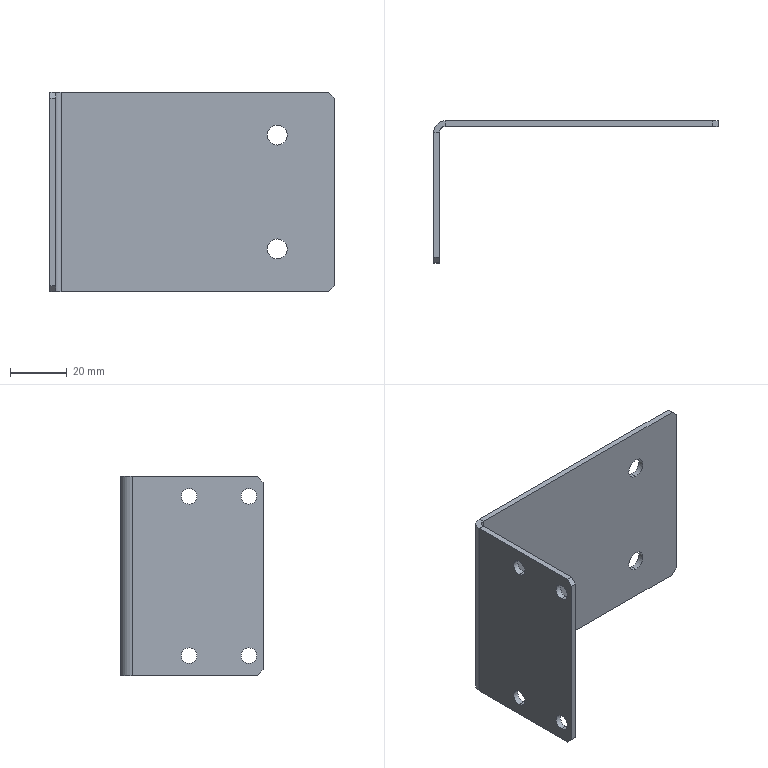Part | NX | features BREP 1 | 1 solid | 30 faces | box 100 x 50 x 70 mm | volume 20180 mm3 | plane 16 | cylinder 14 | commonest cylinder face diameters 5.5 x8 7 x4 4 x1 8 x1
STEP:
#1=CARTESIAN_POINT('',(-98.,-50.,-33.));
#2=VERTEX_POINT('',#1);
#3=CARTESIAN_POINT('',(-98.,-48.,-35.));
#4=VERTEX_POINT('',#3);
#5=CARTESIAN_POINT('',(-98.,-59.,-24.));
#6=DIRECTION('',(0.,0.7071,-0.7071));
#7=VECTOR('',#6,1000.);
#8=LINE('',#5,#7);
#9=EDGE_CURVE('',#2,#4,#8,.T.);
#10=ORIENTED_EDGE('',*,*,#9,.F.);
#11=CARTESIAN_POINT('',(-100.,-50.,-33.));
#12=VERTEX_POINT('',#11);
#13=CARTESIAN_POINT('',(-98.,-50.,-33.));
#14=DIRECTION('',(1.,0.,0.));
#15=VECTOR('',#14,1000.);
#16=LINE('',#13,#15);
#17=EDGE_CURVE('',#12,#2,#16,.T.);
#18=ORIENTED_EDGE('',*,*,#17,.F.);
#19=CARTESIAN_POINT('',(-100.,-48.,-35.));
#20=VERTEX_POINT('',#19);
#21=CARTESIAN_POINT('',(-100.,-48.,-35.));
#22=DIRECTION('',(0.,-0.7071,0.7071));
#23=VECTOR('',#22,1000.);
#24=LINE('',#21,#23);
#25=EDGE_CURVE('',#20,#12,#24,.T.);
#26=ORIENTED_EDGE('',*,*,#25,.F.);
#27=CARTESIAN_POINT('',(-96.,-48.,-35.));
#28=DIRECTION('',(-1.,0.,0.));
#29=VECTOR('',#28,1000.);
#30=LINE('',#27,#29);
#31=EDGE_CURVE('',#4,#20,#30,.T.);
#32=ORIENTED_EDGE('',*,*,#31,.F.);
#33=EDGE_LOOP('',(#10,#18,#26,#32));
#34=FACE_BOUND('',#33,.T.);
#35=CARTESIAN_POINT('',(-96.,-48.,-35.));
#36=DIRECTION('',(0.,0.7071,0.7071));
#37=DIRECTION('',(-1.,0.,0.));
#38=AXIS2_PLACEMENT_3D('',#35,#36,#37);
#39=PLANE('',#38);
#40=ADVANCED_FACE('',(#34),#39,.F.);
#41=CARTESIAN_POINT('',(-98.,-48.,35.));
#42=VERTEX_POINT('',#41);
#43=CARTESIAN_POINT('',(-98.,-50.,33.));
#44=VERTEX_POINT('',#43);
#45=CARTESIAN_POINT('',(-98.,-24.,59.));
#46=DIRECTION('',(0.,-0.7071,-0.7071));
#47=VECTOR('',#46,1000.);
#48=LINE('',#45,#47);
#49=EDGE_CURVE('',#42,#44,#48,.T.);
#50=ORIENTED_EDGE('',*,*,#49,.F.);
#51=CARTESIAN_POINT('',(-100.,-48.,35.));
#52=VERTEX_POINT('',#51);
#53=CARTESIAN_POINT('',(-96.,-48.,35.));
#54=DIRECTION('',(1.,0.,0.));
#55=VECTOR('',#54,1000.);
#56=LINE('',#53,#55);
#57=EDGE_CURVE('',#52,#42,#56,.T.);
#58=ORIENTED_EDGE('',*,*,#57,.F.);
#59=CARTESIAN_POINT('',(-100.,-50.,33.));
#60=VERTEX_POINT('',#59);
#61=CARTESIAN_POINT('',(-100.,-50.,33.));
#62=DIRECTION('',(0.,0.7071,0.7071));
#63=VECTOR('',#62,1000.);
#64=LINE('',#61,#63);
#65=EDGE_CURVE('',#60,#52,#64,.T.);
#66=ORIENTED_EDGE('',*,*,#65,.F.);
#67=CARTESIAN_POINT('',(-98.,-50.,33.));
#68=DIRECTION('',(-1.,0.,0.));
#69=VECTOR('',#68,1000.);
#70=LINE('',#67,#69);
#71=EDGE_CURVE('',#44,#60,#70,.T.);
#72=ORIENTED_EDGE('',*,*,#71,.F.);
#73=EDGE_LOOP('',(#50,#58,#66,#72));
#74=FACE_BOUND('',#73,.T.);
#75=CARTESIAN_POINT('',(-98.,-50.,33.));
#76=DIRECTION('',(0.,0.7071,-0.7071));
#77=DIRECTION('',(-1.,0.,0.));
#78=AXIS2_PLACEMENT_3D('',#75,#76,#77);
#79=PLANE('',#78);
#80=ADVANCED_FACE('',(#74),#79,.F.);
#81=CARTESIAN_POINT('',(0.,0.,-33.));
#82=VERTEX_POINT('',#81);
#83=CARTESIAN_POINT('',(-2.,0.,-35.));
#84=VERTEX_POINT('',#83);
#85=CARTESIAN_POINT('',(-2.,0.,-35.));
#86=DIRECTION('',(-0.7071,0.,-0.7071));
#87=VECTOR('',#86,1000.);
#88=LINE('',#85,#87);
#89=EDGE_CURVE('',#82,#84,#88,.T.);
#90=ORIENTED_EDGE('',*,*,#89,.F.);
#91=CARTESIAN_POINT('',(0.,-2.,-33.));
#92=VERTEX_POINT('',#91);
#93=CARTESIAN_POINT('',(0.,0.,-33.));
#94=DIRECTION('',(0.,1.,0.));
#95=VECTOR('',#94,1000.);
#96=LINE('',#93,#95);
#97=EDGE_CURVE('',#92,#82,#96,.T.);
#98=ORIENTED_EDGE('',*,*,#97,.F.);
#99=CARTESIAN_POINT('',(-2.,-2.,-35.));
#100=VERTEX_POINT('',#99);
#101=CARTESIAN_POINT('',(34.,-2.,1.));
#102=DIRECTION('',(0.7071,0.,0.7071));
#103=VECTOR('',#102,1000.);
#104=LINE('',#101,#103);
#105=EDGE_CURVE('',#100,#92,#104,.T.);
#106=ORIENTED_EDGE('',*,*,#105,.F.);
#107=CARTESIAN_POINT('',(-2.,-2.,-35.));
#108=DIRECTION('',(0.,-1.,0.));
#109=VECTOR('',#108,1000.);
#110=LINE('',#107,#109);
#111=EDGE_CURVE('',#84,#100,#110,.T.);
#112=ORIENTED_EDGE('',*,*,#111,.F.);
#113=EDGE_LOOP('',(#90,#98,#106,#112));
#114=FACE_BOUND('',#113,.T.);
#115=CARTESIAN_POINT('',(-2.,-4.,-35.));
#116=DIRECTION('',(0.7071,0.,-0.7071));
#117=DIRECTION('',(0.,1.,0.));
#118=AXIS2_PLACEMENT_3D('',#115,#116,#117);
#119=PLANE('',#118);
#120=ADVANCED_FACE('',(#114),#119,.T.);
#121=CARTESIAN_POINT('',(-2.,0.,35.));
#122=VERTEX_POINT('',#121);
#123=CARTESIAN_POINT('',(0.,0.,33.));
#124=VERTEX_POINT('',#123);
#125=CARTESIAN_POINT('',(0.,0.,33.));
#126=DIRECTION('',(0.7071,0.,-0.7071));
#127=VECTOR('',#126,1000.);
#128=LINE('',#125,#127);
#129=EDGE_CURVE('',#122,#124,#128,.T.);
#130=ORIENTED_EDGE('',*,*,#129,.F.);
#131=CARTESIAN_POINT('',(-2.,-2.,35.));
#132=VERTEX_POINT('',#131);
#133=CARTESIAN_POINT('',(-2.,-4.,35.));
#134=DIRECTION('',(0.,1.,0.));
#135=VECTOR('',#134,1000.);
#136=LINE('',#133,#135);
#137=EDGE_CURVE('',#132,#122,#136,.T.);
#138=ORIENTED_EDGE('',*,*,#137,.F.);
#139=CARTESIAN_POINT('',(0.,-2.,33.));
#140=VERTEX_POINT('',#139);
#141=CARTESIAN_POINT('',(-1.,-2.,34.));
#142=DIRECTION('',(-0.7071,0.,0.7071));
#143=VECTOR('',#142,1000.);
#144=LINE('',#141,#143);
#145=EDGE_CURVE('',#140,#132,#144,.T.);
#146=ORIENTED_EDGE('',*,*,#145,.F.);
#147=CARTESIAN_POINT('',(0.,0.,33.));
#148=DIRECTION('',(0.,-1.,0.));
#149=VECTOR('',#148,1000.);
#150=LINE('',#147,#149);
#151=EDGE_CURVE('',#124,#140,#150,.T.);
#152=ORIENTED_EDGE('',*,*,#151,.F.);
#153=EDGE_LOOP('',(#130,#138,#146,#152));
#154=FACE_BOUND('',#153,.T.);
#155=CARTESIAN_POINT('',(0.,0.,33.));
#156=DIRECTION('',(-0.7071,0.,-0.7071));
#157=DIRECTION('',(0.,-1.,0.));
#158=AXIS2_PLACEMENT_3D('',#155,#156,#157);
#159=PLANE('',#158);
#160=ADVANCED_FACE('',(#154),#159,.F.);
#161=CARTESIAN_POINT('',(-20.,0.,-23.5));
#162=VERTEX_POINT('',#161);
#163=CARTESIAN_POINT('',(-20.,-2.,-23.5));
#164=VERTEX_POINT('',#163);
#165=CARTESIAN_POINT('',(-20.,0.,-23.5));
#166=DIRECTION('',(0.,1.,0.));
#167=VECTOR('',#166,1000.);
#168=LINE('',#165,#167);
#169=EDGE_CURVE('',#162,#164,#168,.F.);
#170=ORIENTED_EDGE('',*,*,#169,.T.);
#171=CARTESIAN_POINT('',(-20.,-2.,-16.5));
#172=VERTEX_POINT('',#171);
#173=CARTESIAN_POINT('',(-20.,-2.,-20.));
#174=DIRECTION('',(0.,-1.,0.));
#175=DIRECTION('',(1.,0.,0.));
#176=AXIS2_PLACEMENT_3D('',#173,#174,#175);
#177=CIRCLE('',#176,3.5);
#178=EDGE_CURVE('',#164,#172,#177,.T.);
#179=ORIENTED_EDGE('',*,*,#178,.T.);
#180=CARTESIAN_POINT('',(-20.,0.,-16.5));
#181=VERTEX_POINT('',#180);
#182=CARTESIAN_POINT('',(-20.,0.,-16.5));
#183=DIRECTION('',(0.,1.,0.));
#184=VECTOR('',#183,1000.);
#185=LINE('',#182,#184);
#186=EDGE_CURVE('',#181,#172,#185,.F.);
#187=ORIENTED_EDGE('',*,*,#186,.F.);
#188=CARTESIAN_POINT('',(-20.,0.,-20.));
#189=DIRECTION('',(0.,1.,0.));
#190=DIRECTION('',(0.,0.,1.));
#191=AXIS2_PLACEMENT_3D('',#188,#189,#190);
#192=CIRCLE('',#191,3.5);
#193=EDGE_CURVE('',#181,#162,#192,.T.);
#194=ORIENTED_EDGE('',*,*,#193,.T.);
#195=EDGE_LOOP('',(#170,#179,#187,#194));
#196=FACE_BOUND('',#195,.T.);
#197=CARTESIAN_POINT('',(-20.,0.,-20.));
#198=DIRECTION('',(0.,1.,0.));
#199=DIRECTION('',(0.,0.,1.));
#200=AXIS2_PLACEMENT_3D('',#197,#198,#199);
#201=CYLINDRICAL_SURFACE('',#200,3.5);
#202=ADVANCED_FACE('',(#196),#201,.F.);
#203=CARTESIAN_POINT('',(-20.,0.,16.5));
#204=VERTEX_POINT('',#203);
#205=CARTESIAN_POINT('',(-20.,-2.,16.5));
#206=VERTEX_POINT('',#205);
#207=CARTESIAN_POINT('',(-20.,0.,16.5));
#208=DIRECTION('',(0.,1.,0.));
#209=VECTOR('',#208,1000.);
#210=LINE('',#207,#209);
#211=EDGE_CURVE('',#204,#206,#210,.F.);
#212=ORIENTED_EDGE('',*,*,#211,.T.);
#213=CARTESIAN_POINT('',(-20.,-2.,23.5));
#214=VERTEX_POINT('',#213);
#215=CARTESIAN_POINT('',(-20.,-2.,20.));
#216=DIRECTION('',(0.,-1.,0.));
#217=DIRECTION('',(1.,0.,0.));
#218=AXIS2_PLACEMENT_3D('',#215,#216,#217);
#219=CIRCLE('',#218,3.5);
#220=EDGE_CURVE('',#206,#214,#219,.T.);
#221=ORIENTED_EDGE('',*,*,#220,.T.);
#222=CARTESIAN_POINT('',(-20.,0.,23.5));
#223=VERTEX_POINT('',#222);
#224=CARTESIAN_POINT('',(-20.,0.,23.5));
#225=DIRECTION('',(0.,1.,0.));
#226=VECTOR('',#225,1000.);
#227=LINE('',#224,#226);
#228=EDGE_CURVE('',#223,#214,#227,.F.);
#229=ORIENTED_EDGE('',*,*,#228,.F.);
#230=CARTESIAN_POINT('',(-20.,0.,20.));
#231=DIRECTION('',(0.,1.,0.));
#232=DIRECTION('',(0.,0.,1.));
#233=AXIS2_PLACEMENT_3D('',#230,#231,#232);
#234=CIRCLE('',#233,3.5);
#235=EDGE_CURVE('',#223,#204,#234,.T.);
#236=ORIENTED_EDGE('',*,*,#235,.T.);
#237=EDGE_LOOP('',(#212,#221,#229,#236));
#238=FACE_BOUND('',#237,.T.);
#239=CARTESIAN_POINT('',(-20.,0.,20.));
#240=DIRECTION('',(0.,1.,0.));
#241=DIRECTION('',(0.,0.,1.));
#242=AXIS2_PLACEMENT_3D('',#239,#240,#241);
#243=CYLINDRICAL_SURFACE('',#242,3.5);
#244=ADVANCED_FACE('',(#238),#243,.F.);
#245=CARTESIAN_POINT('',(-100.,-24.,-30.75));
#246=VERTEX_POINT('',#245);
#247=CARTESIAN_POINT('',(-98.,-24.,-30.75));
#248=VERTEX_POINT('',#247);
#249=CARTESIAN_POINT('',(-100.,-24.,-30.75));
#250=DIRECTION('',(-1.,0.,0.));
#251=VECTOR('',#250,1000.);
#252=LINE('',#249,#251);
#253=EDGE_CURVE('',#246,#248,#252,.F.);
#254=ORIENTED_EDGE('',*,*,#253,.T.);
#255=CARTESIAN_POINT('',(-98.,-24.,-25.25));
#256=VERTEX_POINT('',#255);
#257=CARTESIAN_POINT('',(-98.,-24.,-28.));
#258=DIRECTION('',(1.,0.,0.));
#259=DIRECTION('',(0.,0.,-1.));
#260=AXIS2_PLACEMENT_3D('',#257,#258,#259);
#261=CIRCLE('',#260,2.75);
#262=EDGE_CURVE('',#248,#256,#261,.T.);
#263=ORIENTED_EDGE('',*,*,#262,.T.);
#264=CARTESIAN_POINT('',(-100.,-24.,-25.25));
#265=VERTEX_POINT('',#264);
#266=CARTESIAN_POINT('',(-100.,-24.,-25.25));
#267=DIRECTION('',(-1.,0.,0.));
#268=VECTOR('',#267,1000.);
#269=LINE('',#266,#268);
#270=EDGE_CURVE('',#265,#256,#269,.F.);
#271=ORIENTED_EDGE('',*,*,#270,.F.);
#272=CARTESIAN_POINT('',(-100.,-24.,-28.));
#273=DIRECTION('',(-1.,0.,0.));
#274=DIRECTION('',(0.,0.,1.));
#275=AXIS2_PLACEMENT_3D('',#272,#273,#274);
#276=CIRCLE('',#275,2.75);
#277=EDGE_CURVE('',#265,#246,#276,.T.);
#278=ORIENTED_EDGE('',*,*,#277,.T.);
#279=EDGE_LOOP('',(#254,#263,#271,#278));
#280=FACE_BOUND('',#279,.T.);
#281=CARTESIAN_POINT('',(-100.,-24.,-28.));
#282=DIRECTION('',(-1.,0.,0.));
#283=DIRECTION('',(0.,0.,1.));
#284=AXIS2_PLACEMENT_3D('',#281,#282,#283);
#285=CYLINDRICAL_SURFACE('',#284,2.75);
#286=ADVANCED_FACE('',(#280),#285,.F.);
#287=CARTESIAN_POINT('',(-100.,-24.,25.25));
#288=VERTEX_POINT('',#287);
#289=CARTESIAN_POINT('',(-98.,-24.,25.25));
#290=VERTEX_POINT('',#289);
#291=CARTESIAN_POINT('',(-100.,-24.,25.25));
#292=DIRECTION('',(-1.,0.,0.));
#293=VECTOR('',#292,1000.);
#294=LINE('',#291,#293);
#295=EDGE_CURVE('',#288,#290,#294,.F.);
#296=ORIENTED_EDGE('',*,*,#295,.T.);
#297=CARTESIAN_POINT('',(-98.,-24.,30.75));
#298=VERTEX_POINT('',#297);
#299=CARTESIAN_POINT('',(-98.,-24.,28.));
#300=DIRECTION('',(1.,0.,0.));
#301=DIRECTION('',(0.,0.,-1.));
#302=AXIS2_PLACEMENT_3D('',#299,#300,#301);
#303=CIRCLE('',#302,2.75);
#304=EDGE_CURVE('',#290,#298,#303,.T.);
#305=ORIENTED_EDGE('',*,*,#304,.T.);
#306=CARTESIAN_POINT('',(-100.,-24.,30.75));
#307=VERTEX_POINT('',#306);
#308=CARTESIAN_POINT('',(-100.,-24.,30.75));
#309=DIRECTION('',(-1.,0.,0.));
#310=VECTOR('',#309,1000.);
#311=LINE('',#308,#310);
#312=EDGE_CURVE('',#307,#298,#311,.F.);
#313=ORIENTED_EDGE('',*,*,#312,.F.);
#314=CARTESIAN_POINT('',(-100.,-24.,28.));
#315=DIRECTION('',(-1.,0.,0.));
#316=DIRECTION('',(0.,0.,1.));
#317=AXIS2_PLACEMENT_3D('',#314,#315,#316);
#318=CIRCLE('',#317,2.75);
#319=EDGE_CURVE('',#307,#288,#318,.T.);
#320=ORIENTED_EDGE('',*,*,#319,.T.);
#321=EDGE_LOOP('',(#296,#305,#313,#320));
#322=FACE_BOUND('',#321,.T.);
#323=CARTESIAN_POINT('',(-100.,-24.,28.));
#324=DIRECTION('',(-1.,0.,0.));
#325=DIRECTION('',(0.,0.,1.));
#326=AXIS2_PLACEMENT_3D('',#323,#324,#325);
#327=CYLINDRICAL_SURFACE('',#326,2.75);
#328=ADVANCED_FACE('',(#322),#327,.F.);
#329=CARTESIAN_POINT('',(-100.,-45.,-30.75));
#330=VERTEX_POINT('',#329);
#331=CARTESIAN_POINT('',(-98.,-45.,-30.75));
#332=VERTEX_POINT('',#331);
#333=CARTESIAN_POINT('',(-100.,-45.,-30.75));
#334=DIRECTION('',(-1.,0.,0.));
#335=VECTOR('',#334,1000.);
#336=LINE('',#333,#335);
#337=EDGE_CURVE('',#330,#332,#336,.F.);
#338=ORIENTED_EDGE('',*,*,#337,.T.);
#339=CARTESIAN_POINT('',(-98.,-45.,-25.25));
#340=VERTEX_POINT('',#339);
#341=CARTESIAN_POINT('',(-98.,-45.,-28.));
#342=DIRECTION('',(1.,0.,0.));
#343=DIRECTION('',(0.,0.,-1.));
#344=AXIS2_PLACEMENT_3D('',#341,#342,#343);
#345=CIRCLE('',#344,2.75);
#346=EDGE_CURVE('',#332,#340,#345,.T.);
#347=ORIENTED_EDGE('',*,*,#346,.T.);
#348=CARTESIAN_POINT('',(-100.,-45.,-25.25));
#349=VERTEX_POINT('',#348);
#350=CARTESIAN_POINT('',(-100.,-45.,-25.25));
#351=DIRECTION('',(-1.,0.,0.));
#352=VECTOR('',#351,1000.);
#353=LINE('',#350,#352);
#354=EDGE_CURVE('',#349,#340,#353,.F.);
#355=ORIENTED_EDGE('',*,*,#354,.F.);
#356=CARTESIAN_POINT('',(-100.,-45.,-28.));
#357=DIRECTION('',(-1.,0.,0.));
#358=DIRECTION('',(0.,0.,1.));
#359=AXIS2_PLACEMENT_3D('',#356,#357,#358);
#360=CIRCLE('',#359,2.75);
#361=EDGE_CURVE('',#349,#330,#360,.T.);
#362=ORIENTED_EDGE('',*,*,#361,.T.);
#363=EDGE_LOOP('',(#338,#347,#355,#362));
#364=FACE_BOUND('',#363,.T.);
#365=CARTESIAN_POINT('',(-100.,-45.,-28.));
#366=DIRECTION('',(-1.,0.,0.));
#367=DIRECTION('',(0.,0.,1.));
#368=AXIS2_PLACEMENT_3D('',#365,#366,#367);
#369=CYLINDRICAL_SURFACE('',#368,2.75);
#370=ADVANCED_FACE('',(#364),#369,.F.);
#371=CARTESIAN_POINT('',(-100.,-45.,25.25));
#372=VERTEX_POINT('',#371);
#373=CARTESIAN_POINT('',(-98.,-45.,25.25));
#374=VERTEX_POINT('',#373);
#375=CARTESIAN_POINT('',(-100.,-45.,25.25));
#376=DIRECTION('',(-1.,0.,0.));
#377=VECTOR('',#376,1000.);
#378=LINE('',#375,#377);
#379=EDGE_CURVE('',#372,#374,#378,.F.);
#380=ORIENTED_EDGE('',*,*,#379,.T.);
#381=CARTESIAN_POINT('',(-98.,-45.,30.75));
#382=VERTEX_POINT('',#381);
#383=CARTESIAN_POINT('',(-98.,-45.,28.));
#384=DIRECTION('',(1.,0.,0.));
#385=DIRECTION('',(0.,0.,-1.));
#386=AXIS2_PLACEMENT_3D('',#383,#384,#385);
#387=CIRCLE('',#386,2.75);
#388=EDGE_CURVE('',#374,#382,#387,.T.);
#389=ORIENTED_EDGE('',*,*,#388,.T.);
#390=CARTESIAN_POINT('',(-100.,-45.,30.75));
#391=VERTEX_POINT('',#390);
#392=CARTESIAN_POINT('',(-100.,-45.,30.75));
#393=DIRECTION('',(-1.,0.,0.));
#394=VECTOR('',#393,1000.);
#395=LINE('',#392,#394);
#396=EDGE_CURVE('',#391,#382,#395,.F.);
#397=ORIENTED_EDGE('',*,*,#396,.F.);
#398=CARTESIAN_POINT('',(-100.,-45.,28.));
#399=DIRECTION('',(-1.,0.,0.));
#400=DIRECTION('',(0.,0.,1.));
#401=AXIS2_PLACEMENT_3D('',#398,#399,#400);
#402=CIRCLE('',#401,2.75);
#403=EDGE_CURVE('',#391,#372,#402,.T.);
#404=ORIENTED_EDGE('',*,*,#403,.T.);
#405=EDGE_LOOP('',(#380,#389,#397,#404));
#406=FACE_BOUND('',#405,.T.);
#407=CARTESIAN_POINT('',(-100.,-45.,28.));
#408=DIRECTION('',(-1.,0.,0.));
#409=DIRECTION('',(0.,0.,1.));
#410=AXIS2_PLACEMENT_3D('',#407,#408,#409);
#411=CYLINDRICAL_SURFACE('',#410,2.75);
#412=ADVANCED_FACE('',(#406),#411,.F.);
#413=CARTESIAN_POINT('',(-96.,0.,-35.));
#414=VERTEX_POINT('',#413);
#415=CARTESIAN_POINT('',(0.,0.,-35.));
#416=DIRECTION('',(-1.,0.,0.));
#417=VECTOR('',#416,1000.);
#418=LINE('',#415,#417);
#419=EDGE_CURVE('',#84,#414,#418,.T.);
#420=ORIENTED_EDGE('',*,*,#419,.F.);
#421=ORIENTED_EDGE('',*,*,#111,.T.);
#422=CARTESIAN_POINT('',(-96.,-2.,-35.));
#423=VERTEX_POINT('',#422);
#424=CARTESIAN_POINT('',(0.,-2.,-35.));
#425=DIRECTION('',(-1.,0.,0.));
#426=VECTOR('',#425,1000.);
#427=LINE('',#424,#426);
#428=EDGE_CURVE('',#100,#423,#427,.T.);
#429=ORIENTED_EDGE('',*,*,#428,.T.);
#430=CARTESIAN_POINT('',(-96.,-2.,-35.));
#431=DIRECTION('',(0.,1.,0.));
#432=VECTOR('',#431,1000.);
#433=LINE('',#430,#432);
#434=EDGE_CURVE('',#423,#414,#433,.T.);
#435=ORIENTED_EDGE('',*,*,#434,.T.);
#436=EDGE_LOOP('',(#420,#421,#429,#435));
#437=FACE_BOUND('',#436,.T.);
#438=CARTESIAN_POINT('',(-96.,-4.,-35.));
#439=DIRECTION('',(0.,0.,1.));
#440=DIRECTION('',(1.,0.,0.));
#441=AXIS2_PLACEMENT_3D('',#438,#439,#440);
#442=PLANE('',#441);
#443=ADVANCED_FACE('',(#437),#442,.F.);
#444=CARTESIAN_POINT('',(-100.,-4.,35.));
#445=VERTEX_POINT('',#444);
#446=CARTESIAN_POINT('',(-100.,0.,35.));
#447=DIRECTION('',(0.,-1.,0.));
#448=VECTOR('',#447,1000.);
#449=LINE('',#446,#448);
#450=EDGE_CURVE('',#445,#52,#449,.T.);
#451=ORIENTED_EDGE('',*,*,#450,.T.);
#452=ORIENTED_EDGE('',*,*,#57,.T.);
#453=CARTESIAN_POINT('',(-98.,-4.,35.));
#454=VERTEX_POINT('',#453);
#455=CARTESIAN_POINT('',(-98.,0.,35.));
#456=DIRECTION('',(0.,-1.,0.));
#457=VECTOR('',#456,1000.);
#458=LINE('',#455,#457);
#459=EDGE_CURVE('',#454,#42,#458,.T.);
#460=ORIENTED_EDGE('',*,*,#459,.F.);
#461=CARTESIAN_POINT('',(-98.,-4.,35.));
#462=DIRECTION('',(-1.,0.,0.));
#463=VECTOR('',#462,1000.);
#464=LINE('',#461,#463);
#465=EDGE_CURVE('',#454,#445,#464,.T.);
#466=ORIENTED_EDGE('',*,*,#465,.T.);
#467=EDGE_LOOP('',(#451,#452,#460,#466));
#468=FACE_BOUND('',#467,.T.);
#469=CARTESIAN_POINT('',(-96.,-4.,35.));
#470=DIRECTION('',(0.,0.,1.));
#471=DIRECTION('',(1.,0.,0.));
#472=AXIS2_PLACEMENT_3D('',#469,#470,#471);
#473=PLANE('',#472);
#474=ADVANCED_FACE('',(#468),#473,.T.);
#475=CARTESIAN_POINT('',(-100.,-4.,-35.));
#476=VERTEX_POINT('',#475);
#477=CARTESIAN_POINT('',(-96.,-4.,-35.));
#478=DIRECTION('',(0.,0.,1.));
#479=DIRECTION('',(-1.,0.,0.));
#480=AXIS2_PLACEMENT_3D('',#477,#478,#479);
#481=CIRCLE('',#480,4.);
#482=EDGE_CURVE('',#414,#476,#481,.T.);
#483=ORIENTED_EDGE('',*,*,#482,.T.);
#484=CARTESIAN_POINT('',(-100.,-4.,35.));
#485=DIRECTION('',(0.,0.,-1.));
#486=VECTOR('',#485,1000.);
#487=LINE('',#484,#486);
#488=EDGE_CURVE('',#445,#476,#487,.T.);
#489=ORIENTED_EDGE('',*,*,#488,.F.);
#490=CARTESIAN_POINT('',(-96.,0.,35.));
#491=VERTEX_POINT('',#490);
#492=CARTESIAN_POINT('',(-96.,-4.,35.));
#493=DIRECTION('',(0.,0.,1.));
#494=DIRECTION('',(-1.,0.,0.));
#495=AXIS2_PLACEMENT_3D('',#492,#493,#494);
#496=CIRCLE('',#495,4.);
#497=EDGE_CURVE('',#491,#445,#496,.T.);
#498=ORIENTED_EDGE('',*,*,#497,.F.);
#499=CARTESIAN_POINT('',(-96.,0.,35.));
#500=DIRECTION('',(0.,0.,-1.));
#501=VECTOR('',#500,1000.);
#502=LINE('',#499,#501);
#503=EDGE_CURVE('',#491,#414,#502,.T.);
#504=ORIENTED_EDGE('',*,*,#503,.T.);
#505=EDGE_LOOP('',(#483,#489,#498,#504));
#506=FACE_BOUND('',#505,.T.);
#507=CARTESIAN_POINT('',(-96.,-4.,35.));
#508=DIRECTION('',(0.,0.,-1.));
#509=DIRECTION('',(-1.,0.,0.));
#510=AXIS2_PLACEMENT_3D('',#507,#508,#509);
#511=CYLINDRICAL_SURFACE('',#510,4.);
#512=ADVANCED_FACE('',(#506),#511,.T.);
#513=CARTESIAN_POINT('',(0.,0.,35.));
#514=DIRECTION('',(-1.,0.,0.));
#515=VECTOR('',#514,1000.);
#516=LINE('',#513,#515);
#517=EDGE_CURVE('',#122,#491,#516,.T.);
#518=ORIENTED_EDGE('',*,*,#517,.F.);
#519=ORIENTED_EDGE('',*,*,#129,.T.);
#520=CARTESIAN_POINT('',(0.,0.,35.));
#521=DIRECTION('',(0.,0.,-1.));
#522=VECTOR('',#521,1000.);
#523=LINE('',#520,#522);
#524=EDGE_CURVE('',#124,#82,#523,.T.);
#525=ORIENTED_EDGE('',*,*,#524,.T.);
#526=ORIENTED_EDGE('',*,*,#89,.T.);
#527=ORIENTED_EDGE('',*,*,#419,.T.);
#528=ORIENTED_EDGE('',*,*,#503,.F.);
#529=EDGE_LOOP('',(#518,#519,#525,#526,#527,#528));
#530=FACE_BOUND('',#529,.T.);
#531=ORIENTED_EDGE('',*,*,#235,.F.);
#532=CARTESIAN_POINT('',(-20.,0.,20.));
#533=DIRECTION('',(0.,1.,0.));
#534=DIRECTION('',(0.,0.,1.));
#535=AXIS2_PLACEMENT_3D('',#532,#533,#534);
#536=CIRCLE('',#535,3.5);
#537=EDGE_CURVE('',#204,#223,#536,.T.);
#538=ORIENTED_EDGE('',*,*,#537,.F.);
#539=EDGE_LOOP('',(#531,#538));
#540=FACE_BOUND('',#539,.T.);
#541=ORIENTED_EDGE('',*,*,#193,.F.);
#542=CARTESIAN_POINT('',(-20.,0.,-20.));
#543=DIRECTION('',(0.,1.,0.));
#544=DIRECTION('',(0.,0.,1.));
#545=AXIS2_PLACEMENT_3D('',#542,#543,#544);
#546=CIRCLE('',#545,3.5);
#547=EDGE_CURVE('',#162,#181,#546,.T.);
#548=ORIENTED_EDGE('',*,*,#547,.F.);
#549=EDGE_LOOP('',(#541,#548));
#550=FACE_BOUND('',#549,.T.);
#551=CARTESIAN_POINT('',(0.,0.,35.));
#552=DIRECTION('',(0.,-1.,0.));
#553=DIRECTION('',(1.,0.,0.));
#554=AXIS2_PLACEMENT_3D('',#551,#552,#553);
#555=PLANE('',#554);
#556=ADVANCED_FACE('',(#530,#540,#550),#555,.F.);
#557=ORIENTED_EDGE('',*,*,#524,.F.);
#558=ORIENTED_EDGE('',*,*,#151,.T.);
#559=CARTESIAN_POINT('',(0.,-2.,35.));
#560=DIRECTION('',(0.,0.,-1.));
#561=VECTOR('',#560,1000.);
#562=LINE('',#559,#561);
#563=EDGE_CURVE('',#140,#92,#562,.T.);
#564=ORIENTED_EDGE('',*,*,#563,.T.);
#565=ORIENTED_EDGE('',*,*,#97,.T.);
#566=EDGE_LOOP('',(#557,#558,#564,#565));
#567=FACE_BOUND('',#566,.T.);
#568=CARTESIAN_POINT('',(0.,0.,35.));
#569=DIRECTION('',(1.,0.,0.));
#570=DIRECTION('',(0.,1.,0.));
#571=AXIS2_PLACEMENT_3D('',#568,#569,#570);
#572=PLANE('',#571);
#573=ADVANCED_FACE('',(#567),#572,.T.);
#574=ORIENTED_EDGE('',*,*,#563,.F.);
#575=ORIENTED_EDGE('',*,*,#145,.T.);
#576=CARTESIAN_POINT('',(-96.,-2.,35.));
#577=VERTEX_POINT('',#576);
#578=CARTESIAN_POINT('',(0.,-2.,35.));
#579=DIRECTION('',(-1.,0.,0.));
#580=VECTOR('',#579,1000.);
#581=LINE('',#578,#580);
#582=EDGE_CURVE('',#132,#577,#581,.T.);
#583=ORIENTED_EDGE('',*,*,#582,.T.);
#584=CARTESIAN_POINT('',(-96.,-2.,35.));
#585=DIRECTION('',(0.,0.,-1.));
#586=VECTOR('',#585,1000.);
#587=LINE('',#584,#586);
#588=EDGE_CURVE('',#577,#423,#587,.T.);
#589=ORIENTED_EDGE('',*,*,#588,.T.);
#590=ORIENTED_EDGE('',*,*,#428,.F.);
#591=ORIENTED_EDGE('',*,*,#105,.T.);
#592=EDGE_LOOP('',(#574,#575,#583,#589,#590,#591));
#593=FACE_BOUND('',#592,.T.);
#594=CARTESIAN_POINT('',(-20.,-2.,20.));
#595=DIRECTION('',(0.,-1.,0.));
#596=DIRECTION('',(1.,0.,0.));
#597=AXIS2_PLACEMENT_3D('',#594,#595,#596);
#598=CIRCLE('',#597,3.5);
#599=EDGE_CURVE('',#214,#206,#598,.T.);
#600=ORIENTED_EDGE('',*,*,#599,.F.);
#601=ORIENTED_EDGE('',*,*,#220,.F.);
#602=EDGE_LOOP('',(#600,#601));
#603=FACE_BOUND('',#602,.T.);
#604=CARTESIAN_POINT('',(-20.,-2.,-20.));
#605=DIRECTION('',(0.,-1.,0.));
#606=DIRECTION('',(1.,0.,0.));
#607=AXIS2_PLACEMENT_3D('',#604,#605,#606);
#608=CIRCLE('',#607,3.5);
#609=EDGE_CURVE('',#172,#164,#608,.T.);
#610=ORIENTED_EDGE('',*,*,#609,.F.);
#611=ORIENTED_EDGE('',*,*,#178,.F.);
#612=EDGE_LOOP('',(#610,#611));
#613=FACE_BOUND('',#612,.T.);
#614=CARTESIAN_POINT('',(0.,-2.,35.));
#615=DIRECTION('',(0.,-1.,0.));
#616=DIRECTION('',(1.,0.,0.));
#617=AXIS2_PLACEMENT_3D('',#614,#615,#616);
#618=PLANE('',#617);
#619=ADVANCED_FACE('',(#593,#603,#613),#618,.T.);
#620=CARTESIAN_POINT('',(-98.,-4.,-35.));
#621=VERTEX_POINT('',#620);
#622=CARTESIAN_POINT('',(-96.,-4.,-35.));
#623=DIRECTION('',(0.,0.,1.));
#624=DIRECTION('',(1.,0.,0.));
#625=AXIS2_PLACEMENT_3D('',#622,#623,#624);
#626=CIRCLE('',#625,2.);
#627=EDGE_CURVE('',#423,#621,#626,.T.);
#628=ORIENTED_EDGE('',*,*,#627,.F.);
#629=ORIENTED_EDGE('',*,*,#588,.F.);
#630=CARTESIAN_POINT('',(-96.,-4.,35.));
#631=DIRECTION('',(0.,0.,1.));
#632=DIRECTION('',(1.,0.,0.));
#633=AXIS2_PLACEMENT_3D('',#630,#631,#632);
#634=CIRCLE('',#633,2.);
#635=EDGE_CURVE('',#577,#454,#634,.T.);
#636=ORIENTED_EDGE('',*,*,#635,.T.);
#637=CARTESIAN_POINT('',(-98.,-4.,35.));
#638=DIRECTION('',(0.,0.,-1.));
#639=VECTOR('',#638,1000.);
#640=LINE('',#637,#639);
#641=EDGE_CURVE('',#454,#621,#640,.T.);
#642=ORIENTED_EDGE('',*,*,#641,.T.);
#643=EDGE_LOOP('',(#628,#629,#636,#642));
#644=FACE_BOUND('',#643,.T.);
#645=CARTESIAN_POINT('',(-96.,-4.,35.));
#646=DIRECTION('',(0.,0.,-1.));
#647=DIRECTION('',(-1.,0.,0.));
#648=AXIS2_PLACEMENT_3D('',#645,#646,#647);
#649=CYLINDRICAL_SURFACE('',#648,2.);
#650=ADVANCED_FACE('',(#644),#649,.F.);
#651=ORIENTED_EDGE('',*,*,#459,.T.);
#652=ORIENTED_EDGE('',*,*,#49,.T.);
#653=CARTESIAN_POINT('',(-98.,-50.,35.));
#654=DIRECTION('',(0.,0.,-1.));
#655=VECTOR('',#654,1000.);
#656=LINE('',#653,#655);
#657=EDGE_CURVE('',#44,#2,#656,.T.);
#658=ORIENTED_EDGE('',*,*,#657,.T.);
#659=ORIENTED_EDGE('',*,*,#9,.T.);
#660=CARTESIAN_POINT('',(-98.,0.,-35.));
#661=DIRECTION('',(0.,-1.,0.));
#662=VECTOR('',#661,1000.);
#663=LINE('',#660,#662);
#664=EDGE_CURVE('',#621,#4,#663,.T.);
#665=ORIENTED_EDGE('',*,*,#664,.F.);
#666=ORIENTED_EDGE('',*,*,#641,.F.);
#667=EDGE_LOOP('',(#651,#652,#658,#659,#665,#666));
#668=FACE_BOUND('',#667,.T.);
#669=CARTESIAN_POINT('',(-98.,-45.,28.));
#670=DIRECTION('',(1.,0.,0.));
#671=DIRECTION('',(0.,0.,-1.));
#672=AXIS2_PLACEMENT_3D('',#669,#670,#671);
#673=CIRCLE('',#672,2.75);
#674=EDGE_CURVE('',#382,#374,#673,.T.);
#675=ORIENTED_EDGE('',*,*,#674,.F.);
#676=ORIENTED_EDGE('',*,*,#388,.F.);
#677=EDGE_LOOP('',(#675,#676));
#678=FACE_BOUND('',#677,.T.);
#679=CARTESIAN_POINT('',(-98.,-45.,-28.));
#680=DIRECTION('',(1.,0.,0.));
#681=DIRECTION('',(0.,0.,-1.));
#682=AXIS2_PLACEMENT_3D('',#679,#680,#681);
#683=CIRCLE('',#682,2.75);
#684=EDGE_CURVE('',#340,#332,#683,.T.);
#685=ORIENTED_EDGE('',*,*,#684,.F.);
#686=ORIENTED_EDGE('',*,*,#346,.F.);
#687=EDGE_LOOP('',(#685,#686));
#688=FACE_BOUND('',#687,.T.);
#689=CARTESIAN_POINT('',(-98.,-24.,28.));
#690=DIRECTION('',(1.,0.,0.));
#691=DIRECTION('',(0.,0.,-1.));
#692=AXIS2_PLACEMENT_3D('',#689,#690,#691);
#693=CIRCLE('',#692,2.75);
#694=EDGE_CURVE('',#298,#290,#693,.T.);
#695=ORIENTED_EDGE('',*,*,#694,.F.);
#696=ORIENTED_EDGE('',*,*,#304,.F.);
#697=EDGE_LOOP('',(#695,#696));
#698=FACE_BOUND('',#697,.T.);
#699=CARTESIAN_POINT('',(-98.,-24.,-28.));
#700=DIRECTION('',(1.,0.,0.));
#701=DIRECTION('',(0.,0.,-1.));
#702=AXIS2_PLACEMENT_3D('',#699,#700,#701);
#703=CIRCLE('',#702,2.75);
#704=EDGE_CURVE('',#256,#248,#703,.T.);
#705=ORIENTED_EDGE('',*,*,#704,.F.);
#706=ORIENTED_EDGE('',*,*,#262,.F.);
#707=EDGE_LOOP('',(#705,#706));
#708=FACE_BOUND('',#707,.T.);
#709=CARTESIAN_POINT('',(-98.,0.,35.));
#710=DIRECTION('',(1.,0.,0.));
#711=DIRECTION('',(0.,0.,-1.));
#712=AXIS2_PLACEMENT_3D('',#709,#710,#711);
#713=PLANE('',#712);
#714=ADVANCED_FACE('',(#668,#678,#688,#698,#708),#713,.T.);
#715=ORIENTED_EDGE('',*,*,#657,.F.);
#716=ORIENTED_EDGE('',*,*,#71,.T.);
#717=CARTESIAN_POINT('',(-100.,-50.,35.));
#718=DIRECTION('',(0.,0.,-1.));
#719=VECTOR('',#718,1000.);
#720=LINE('',#717,#719);
#721=EDGE_CURVE('',#60,#12,#720,.T.);
#722=ORIENTED_EDGE('',*,*,#721,.T.);
#723=ORIENTED_EDGE('',*,*,#17,.T.);
#724=EDGE_LOOP('',(#715,#716,#722,#723));
#725=FACE_BOUND('',#724,.T.);
#726=CARTESIAN_POINT('',(-98.,-50.,35.));
#727=DIRECTION('',(0.,-1.,0.));
#728=DIRECTION('',(0.,0.,-1.));
#729=AXIS2_PLACEMENT_3D('',#726,#727,#728);
#730=PLANE('',#729);
#731=ADVANCED_FACE('',(#725),#730,.T.);
#732=ORIENTED_EDGE('',*,*,#721,.F.);
#733=ORIENTED_EDGE('',*,*,#65,.T.);
#734=ORIENTED_EDGE('',*,*,#450,.F.);
#735=ORIENTED_EDGE('',*,*,#488,.T.);
#736=CARTESIAN_POINT('',(-100.,0.,-35.));
#737=DIRECTION('',(0.,-1.,0.));
#738=VECTOR('',#737,1000.);
#739=LINE('',#736,#738);
#740=EDGE_CURVE('',#476,#20,#739,.T.);
#741=ORIENTED_EDGE('',*,*,#740,.T.);
#742=ORIENTED_EDGE('',*,*,#25,.T.);
#743=EDGE_LOOP('',(#732,#733,#734,#735,#741,#742));
#744=FACE_BOUND('',#743,.T.);
#745=ORIENTED_EDGE('',*,*,#403,.F.);
#746=CARTESIAN_POINT('',(-100.,-45.,28.));
#747=DIRECTION('',(-1.,0.,0.));
#748=DIRECTION('',(0.,0.,1.));
#749=AXIS2_PLACEMENT_3D('',#746,#747,#748);
#750=CIRCLE('',#749,2.75);
#751=EDGE_CURVE('',#372,#391,#750,.T.);
#752=ORIENTED_EDGE('',*,*,#751,.F.);
#753=EDGE_LOOP('',(#745,#752));
#754=FACE_BOUND('',#753,.T.);
#755=ORIENTED_EDGE('',*,*,#361,.F.);
#756=CARTESIAN_POINT('',(-100.,-45.,-28.));
#757=DIRECTION('',(-1.,0.,0.));
#758=DIRECTION('',(0.,0.,1.));
#759=AXIS2_PLACEMENT_3D('',#756,#757,#758);
#760=CIRCLE('',#759,2.75);
#761=EDGE_CURVE('',#330,#349,#760,.T.);
#762=ORIENTED_EDGE('',*,*,#761,.F.);
#763=EDGE_LOOP('',(#755,#762));
#764=FACE_BOUND('',#763,.T.);
#765=ORIENTED_EDGE('',*,*,#319,.F.);
#766=CARTESIAN_POINT('',(-100.,-24.,28.));
#767=DIRECTION('',(-1.,0.,0.));
#768=DIRECTION('',(0.,0.,1.));
#769=AXIS2_PLACEMENT_3D('',#766,#767,#768);
#770=CIRCLE('',#769,2.75);
#771=EDGE_CURVE('',#288,#307,#770,.T.);
#772=ORIENTED_EDGE('',*,*,#771,.F.);
#773=EDGE_LOOP('',(#765,#772));
#774=FACE_BOUND('',#773,.T.);
#775=ORIENTED_EDGE('',*,*,#277,.F.);
#776=CARTESIAN_POINT('',(-100.,-24.,-28.));
#777=DIRECTION('',(-1.,0.,0.));
#778=DIRECTION('',(0.,0.,1.));
#779=AXIS2_PLACEMENT_3D('',#776,#777,#778);
#780=CIRCLE('',#779,2.75);
#781=EDGE_CURVE('',#246,#265,#780,.T.);
#782=ORIENTED_EDGE('',*,*,#781,.F.);
#783=EDGE_LOOP('',(#775,#782));
#784=FACE_BOUND('',#783,.T.);
#785=CARTESIAN_POINT('',(-100.,0.,35.));
#786=DIRECTION('',(1.,0.,0.));
#787=DIRECTION('',(0.,0.,-1.));
#788=AXIS2_PLACEMENT_3D('',#785,#786,#787);
#789=PLANE('',#788);
#790=ADVANCED_FACE('',(#744,#754,#764,#774,#784),#789,.F.);
#791=ORIENTED_EDGE('',*,*,#664,.T.);
#792=ORIENTED_EDGE('',*,*,#31,.T.);
#793=ORIENTED_EDGE('',*,*,#740,.F.);
#794=CARTESIAN_POINT('',(-100.,-4.,-35.));
#795=DIRECTION('',(1.,0.,0.));
#796=VECTOR('',#795,1000.);
#797=LINE('',#794,#796);
#798=EDGE_CURVE('',#476,#621,#797,.T.);
#799=ORIENTED_EDGE('',*,*,#798,.T.);
#800=EDGE_LOOP('',(#791,#792,#793,#799));
#801=FACE_BOUND('',#800,.T.);
#802=CARTESIAN_POINT('',(-96.,-2.,-35.));
#803=DIRECTION('',(0.,0.,-1.));
#804=DIRECTION('',(-1.,0.,0.));
#805=AXIS2_PLACEMENT_3D('',#802,#803,#804);
#806=PLANE('',#805);
#807=ADVANCED_FACE('',(#801),#806,.T.);
#808=ORIENTED_EDGE('',*,*,#798,.F.);
#809=ORIENTED_EDGE('',*,*,#482,.F.);
#810=ORIENTED_EDGE('',*,*,#434,.F.);
#811=ORIENTED_EDGE('',*,*,#627,.T.);
#812=EDGE_LOOP('',(#808,#809,#810,#811));
#813=FACE_BOUND('',#812,.T.);
#814=CARTESIAN_POINT('',(-100.,-4.,-35.));
#815=DIRECTION('',(0.,0.,-1.));
#816=DIRECTION('',(-1.,0.,0.));
#817=AXIS2_PLACEMENT_3D('',#814,#815,#816);
#818=PLANE('',#817);
#819=ADVANCED_FACE('',(#813),#818,.T.);
#820=ORIENTED_EDGE('',*,*,#582,.F.);
#821=ORIENTED_EDGE('',*,*,#137,.T.);
#822=ORIENTED_EDGE('',*,*,#517,.T.);
#823=CARTESIAN_POINT('',(-96.,0.,35.));
#824=DIRECTION('',(0.,-1.,0.));
#825=VECTOR('',#824,1000.);
#826=LINE('',#823,#825);
#827=EDGE_CURVE('',#491,#577,#826,.T.);
#828=ORIENTED_EDGE('',*,*,#827,.T.);
#829=EDGE_LOOP('',(#820,#821,#822,#828));
#830=FACE_BOUND('',#829,.T.);
#831=CARTESIAN_POINT('',(-98.,-4.,35.));
#832=DIRECTION('',(0.,0.,1.));
#833=DIRECTION('',(1.,0.,0.));
#834=AXIS2_PLACEMENT_3D('',#831,#832,#833);
#835=PLANE('',#834);
#836=ADVANCED_FACE('',(#830),#835,.T.);
#837=ORIENTED_EDGE('',*,*,#827,.F.);
#838=ORIENTED_EDGE('',*,*,#497,.T.);
#839=ORIENTED_EDGE('',*,*,#465,.F.);
#840=ORIENTED_EDGE('',*,*,#635,.F.);
#841=EDGE_LOOP('',(#837,#838,#839,#840));
#842=FACE_BOUND('',#841,.T.);
#843=CARTESIAN_POINT('',(-96.,0.,35.));
#844=DIRECTION('',(0.,0.,1.));
#845=DIRECTION('',(1.,0.,0.));
#846=AXIS2_PLACEMENT_3D('',#843,#844,#845);
#847=PLANE('',#846);
#848=ADVANCED_FACE('',(#842),#847,.T.);
#849=ORIENTED_EDGE('',*,*,#674,.T.);
#850=ORIENTED_EDGE('',*,*,#379,.F.);
#851=ORIENTED_EDGE('',*,*,#751,.T.);
#852=ORIENTED_EDGE('',*,*,#396,.T.);
#853=EDGE_LOOP('',(#849,#850,#851,#852));
#854=FACE_BOUND('',#853,.T.);
#855=CARTESIAN_POINT('',(-100.,-45.,28.));
#856=DIRECTION('',(-1.,0.,0.));
#857=DIRECTION('',(0.,0.,1.));
#858=AXIS2_PLACEMENT_3D('',#855,#856,#857);
#859=CYLINDRICAL_SURFACE('',#858,2.75);
#860=ADVANCED_FACE('',(#854),#859,.F.);
#861=ORIENTED_EDGE('',*,*,#684,.T.);
#862=ORIENTED_EDGE('',*,*,#337,.F.);
#863=ORIENTED_EDGE('',*,*,#761,.T.);
#864=ORIENTED_EDGE('',*,*,#354,.T.);
#865=EDGE_LOOP('',(#861,#862,#863,#864));
#866=FACE_BOUND('',#865,.T.);
#867=CARTESIAN_POINT('',(-100.,-45.,-28.));
#868=DIRECTION('',(-1.,0.,0.));
#869=DIRECTION('',(0.,0.,1.));
#870=AXIS2_PLACEMENT_3D('',#867,#868,#869);
#871=CYLINDRICAL_SURFACE('',#870,2.75);
#872=ADVANCED_FACE('',(#866),#871,.F.);
#873=ORIENTED_EDGE('',*,*,#694,.T.);
#874=ORIENTED_EDGE('',*,*,#295,.F.);
#875=ORIENTED_EDGE('',*,*,#771,.T.);
#876=ORIENTED_EDGE('',*,*,#312,.T.);
#877=EDGE_LOOP('',(#873,#874,#875,#876));
#878=FACE_BOUND('',#877,.T.);
#879=CARTESIAN_POINT('',(-100.,-24.,28.));
#880=DIRECTION('',(-1.,0.,0.));
#881=DIRECTION('',(0.,0.,1.));
#882=AXIS2_PLACEMENT_3D('',#879,#880,#881);
#883=CYLINDRICAL_SURFACE('',#882,2.75);
#884=ADVANCED_FACE('',(#878),#883,.F.);
#885=ORIENTED_EDGE('',*,*,#704,.T.);
#886=ORIENTED_EDGE('',*,*,#253,.F.);
#887=ORIENTED_EDGE('',*,*,#781,.T.);
#888=ORIENTED_EDGE('',*,*,#270,.T.);
#889=EDGE_LOOP('',(#885,#886,#887,#888));
#890=FACE_BOUND('',#889,.T.);
#891=CARTESIAN_POINT('',(-100.,-24.,-28.));
#892=DIRECTION('',(-1.,0.,0.));
#893=DIRECTION('',(0.,0.,1.));
#894=AXIS2_PLACEMENT_3D('',#891,#892,#893);
#895=CYLINDRICAL_SURFACE('',#894,2.75);
#896=ADVANCED_FACE('',(#890),#895,.F.);
#897=ORIENTED_EDGE('',*,*,#599,.T.);
#898=ORIENTED_EDGE('',*,*,#211,.F.);
#899=ORIENTED_EDGE('',*,*,#537,.T.);
#900=ORIENTED_EDGE('',*,*,#228,.T.);
#901=EDGE_LOOP('',(#897,#898,#899,#900));
#902=FACE_BOUND('',#901,.T.);
#903=CARTESIAN_POINT('',(-20.,0.,20.));
#904=DIRECTION('',(0.,1.,0.));
#905=DIRECTION('',(0.,0.,1.));
#906=AXIS2_PLACEMENT_3D('',#903,#904,#905);
#907=CYLINDRICAL_SURFACE('',#906,3.5);
#908=ADVANCED_FACE('',(#902),#907,.F.);
#909=ORIENTED_EDGE('',*,*,#609,.T.);
#910=ORIENTED_EDGE('',*,*,#169,.F.);
#911=ORIENTED_EDGE('',*,*,#547,.T.);
#912=ORIENTED_EDGE('',*,*,#186,.T.);
#913=EDGE_LOOP('',(#909,#910,#911,#912));
#914=FACE_BOUND('',#913,.T.);
#915=CARTESIAN_POINT('',(-20.,0.,-20.));
#916=DIRECTION('',(0.,1.,0.));
#917=DIRECTION('',(0.,0.,1.));
#918=AXIS2_PLACEMENT_3D('',#915,#916,#917);
#919=CYLINDRICAL_SURFACE('',#918,3.5);
#920=ADVANCED_FACE('',(#914),#919,.F.);
#921=CLOSED_SHELL('',(#40,#80,#120,#160,#202,#244,#286,#328,#370,#412,#443,#474,#512,#556,#573,#619,#650,#714,#731,#790,#807,#819,#836,#848,#860,#872,#884,#896,#908,#920));
#922=MANIFOLD_SOLID_BREP('',#921);
#923=(LENGTH_UNIT()NAMED_UNIT(*)SI_UNIT(.MILLI.,.METRE.));
#924=UNCERTAINTY_MEASURE_WITH_UNIT(LENGTH_MEASURE(0.00001),#923,'','');
#925=(NAMED_UNIT(*)PLANE_ANGLE_UNIT()SI_UNIT($,.RADIAN.));
#926=(NAMED_UNIT(*)SI_UNIT($,.STERADIAN.)SOLID_ANGLE_UNIT());
#927=(GEOMETRIC_REPRESENTATION_CONTEXT(3)GLOBAL_UNCERTAINTY_ASSIGNED_CONTEXT((#924))GLOBAL_UNIT_ASSIGNED_CONTEXT((#923,#925,#926))REPRESENTATION_CONTEXT('',''));
#928=ADVANCED_BREP_SHAPE_REPRESENTATION('',(#922),#927);